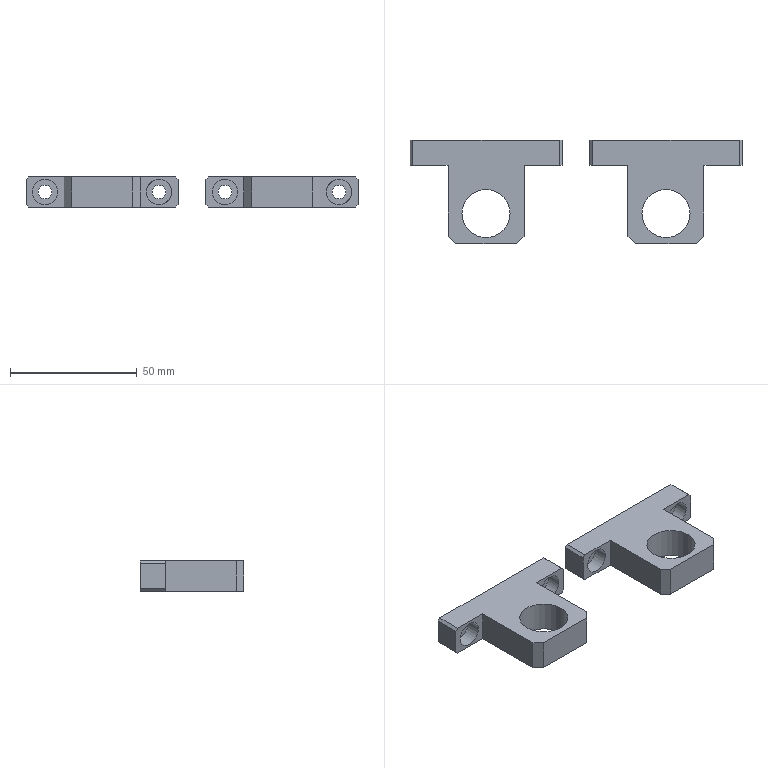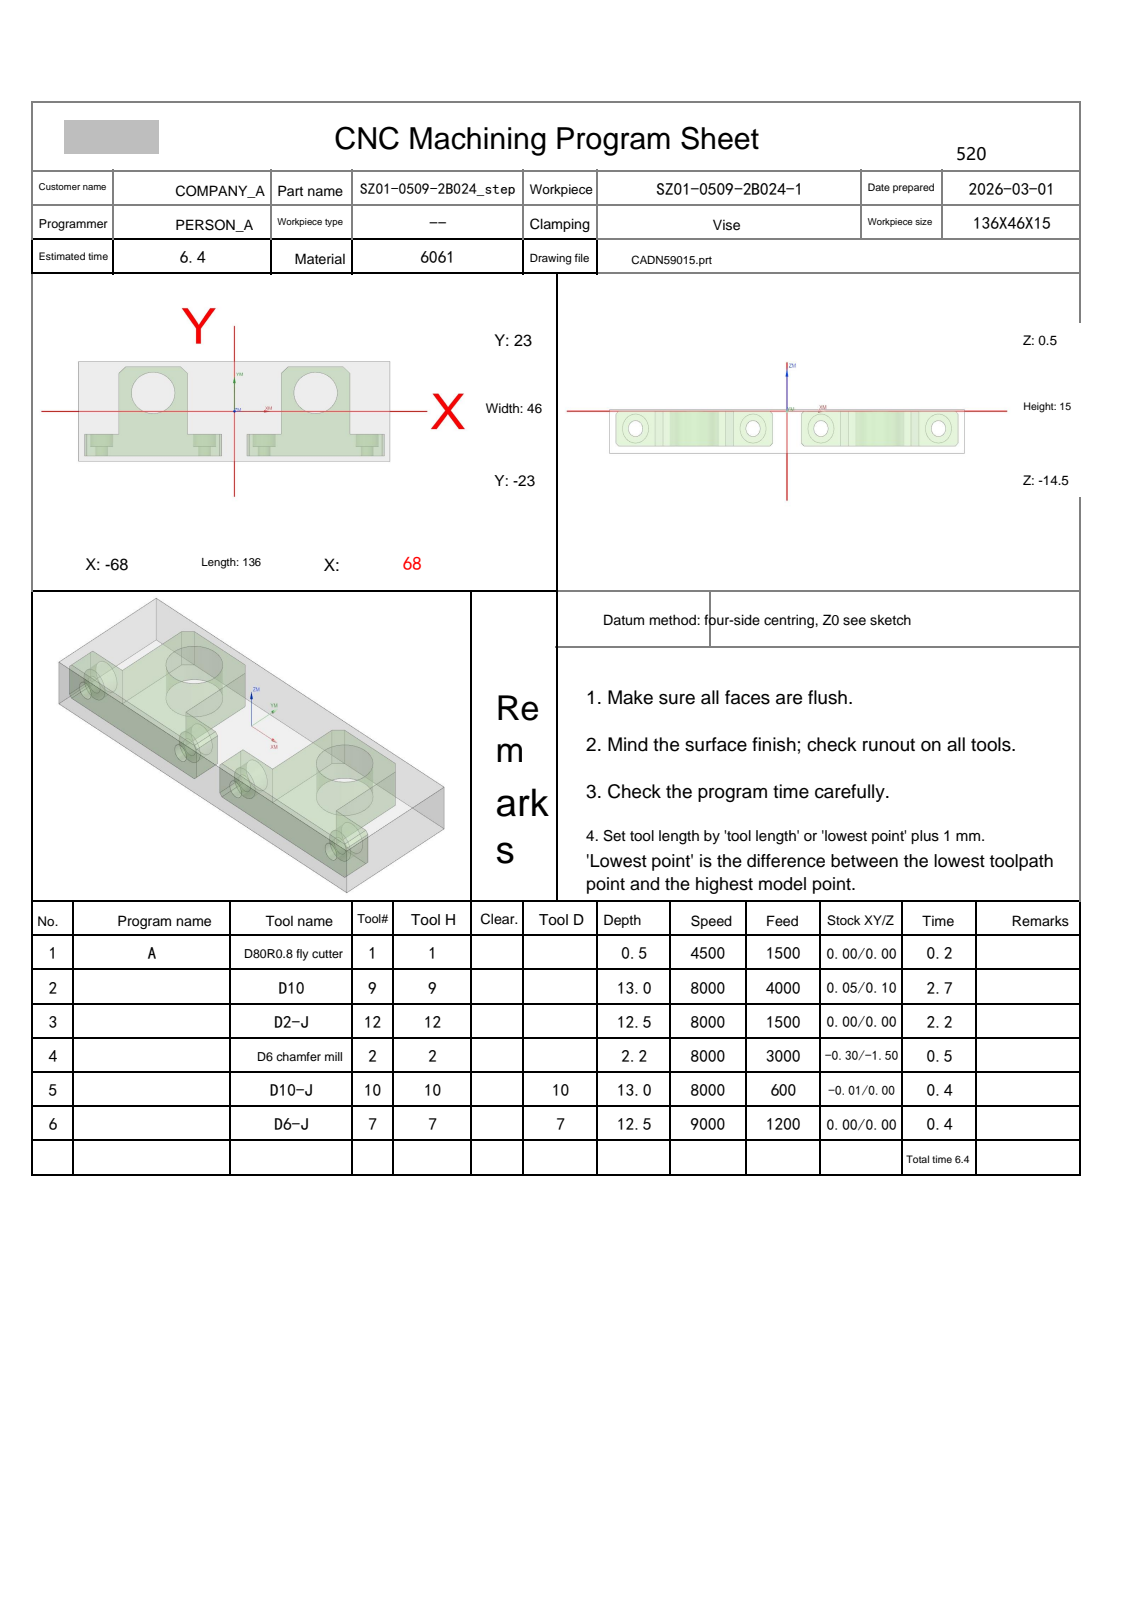NC program | NX | posted by the shop | part box 131 x 41 x 12 mm
Lines 33 to 914 of 8452:
N2 T09 M06
(D10  D=10. R=0. H=09 ce=0.25 di=0.10)
G00 G90 G54 X78.431 Y-9.532 M03 S8000
G43 H09 Z50.
M08
Z-10.
G01 X78.332 Y-9.551 Z-10.625 F4000.
X78.234 Y-9.57 Z-10.872
X78.136 Y-9.588 Z-11.054
X78.038 Y-9.607 Z-11.2
X77.939 Y-9.626 Z-11.323
X77.841 Y-9.644 Z-11.428
X77.743 Y-9.663 Z-11.52
X77.645 Y-9.682 Z-11.6
X77.546 Y-9.7 Z-11.67
X77.448 Y-9.719 Z-11.732
X77.35 Y-9.738 Z-11.786
X77.252 Y-9.756 Z-11.833
X77.153 Y-9.775 Z-11.874
X77.055 Y-9.794 Z-11.908
X76.957 Y-9.812 Z-11.936
X76.859 Y-9.831 Z-11.96
X76.76 Y-9.85 Z-11.977
X76.662 Y-9.869 Z-11.99
X76.564 Y-9.887 Z-11.997
X76.466 Y-9.906 Z-12.
X74.351 Y-10.308
G03 X74. Y-10.567 I.101 J-.505
X73.362 Y-14.375 I12.231 J-4.006
X73.175 Y-21.332 I466.207 J-16.024
G02 X69.942 Y-26.231 I-6.184 J.564
X64.382 Y-27.871 I-6.599 J12.133
X56.567 Y-28.2 I-7.815 J92.472
X55.272 Y-28.191 I0.0 J92.801
G01 X-66.13 Y-28.178
G02 X-71.209 Y-24.969 I.35 J6.178
X-72.866 Y-19.412 I12.012 J6.606
X-73.198 Y-11.704 I89.283 J7.708
X-73.19 Y-10.542 I89.615 J0.0
G01 X-73.178 Y21.13
G02 X-69.969 Y26.209 I6.178 J-.35
X-64.412 Y27.866 I6.606 J-12.012
X-56.704 Y28.198 I7.708 J-89.284
X-55.542 Y28.19 I0.0 J-89.616
G01 X66.15 Y28.176
G02 X71.222 Y24.947 I-.374 J-6.185
X72.868 Y19.389 I-12.074 J-6.599
X73.206 Y11.288 I-97.034 J-8.1
X73.193 Y9.718 I-97.372 J0.0
X73.223 Y2.077 I-972.688 J-7.641
X73.171 Y-8.021 I-972.718 J0.0
G03 X72.526 Y-16.182 I158.167 J-16.601
G01 X72.527 Y-16.395
G02 X72.324 Y-19.878 I-29.998 J0.0
X67.898 Y-25.433 I-7.835 J1.701
X61.268 Y-27.106 I-7.64 J16.307
X51.965 Y-27.41 I-9.303 J141.895
X49.915 Y-27.396 I0.0 J142.199
G01 X-63.987 Y-27.379
G02 X-70.13 Y-23.411 I.587 J7.646
X-72.044 Y-16.849 I14.246 J7.717
X-72.402 Y-8.099 I106.839 J8.75
X-72.392 Y-6.619 I107.197 J0.0
G01 X-72.379 Y18.987
G02 X-68.413 Y25.125 I7.648 J-.591
X-62.168 Y27.003 I7.584 J-13.897
X-53.695 Y27.396 I8.473 J-91.31
X-52.5 Y27.388 I0.0 J-91.702
G01 X63.987 Y27.379
G02 X70.125 Y23.413 I-.591 J-7.648
X72.003 Y17.168 I-13.895 J-7.585
X72.395 Y8.7 I-91.242 J-8.468
X72.388 Y7.5 I-91.635 J0.0
X72.415 Y1.757 I-590.112 J-5.744
X72.352 Y-6.879 I-590.139 J0.0
G03 X71.65 Y-17.634 I789.099 J-56.915
G02 X70.746 Y-20.537 I-9.426 J1.342
G01 X70.57 Y-21.867
X70.045 Y-23.131
X69.211 Y-24.217
X68.124 Y-25.049
X66.859 Y-25.572
G02 X53.023 Y-26.58 I-13.836 J94.442
X52.027 Y-26.575 I0.0 J95.45
G01 X-61.953 Y-26.576
G02 X-65.274 Y-25.768 I.43 J9.002
G01 X-66.859 Y-25.572
X-68.124 Y-25.049
X-69.211 Y-24.217
X-70.045 Y-23.131
X-70.57 Y-21.867
G02 X-71.582 Y-7.951 I95.216 J13.916
X-71.579 Y-7.258 I96.228 J0.0
G01 X-71.575 Y16.961
G02 X-66.822 Y24.292 I8.746 J-.465
X-60.166 Y26.188 I8.154 J-15.995
X-50.795 Y26.602 I9.371 J-105.776
X-49.219 Y26.59 I0.0 J-106.19
G01 X61.968 Y26.575
G02 X69.292 Y21.822 I-.472 J-8.746
X71.177 Y15.251 I-15.881 J-8.113
X71.601 Y5.878 I-103.407 J-9.373
X71.589 Y4.304 I-103.831 J0.0
X71.622 Y.577 I-214.924 J-3.727
X71.462 Y-7.694 I-214.956 J0.0
X70.917 Y-15.927 I-317.939 J16.915
G01 X70.75 Y-16.9
X70.739 Y-20.591
G02 X70.734 Y-17.931 I740.355 J2.66
X70.786 Y-9.213 I740.36 J0.0
G03 X70.973 Y1.153 I-287.439 J10.366
X70.769 Y11.972 I-287.626 J0.0
X69.566 Y19.046 I-25.77 J-.745
X62.385 Y25.338 I-8.77 J-2.765
X55.692 Y25.929 I-6.694 J-37.65
X55.141 Y25.925 I0.0 J-38.24
G01 X49.701 Y25.96
X-50.827 Y25.938
G03 X-51.733 Y25.944 I-.907 J-73.71
X-60.486 Y25.423 I0.0 J-73.716
X-66.63 Y23.268 I1.639 J-14.515
X-70.323 Y17.452 I5.291 J-7.44
X-70.925 Y10.804 I36.408 J-6.648
X-70.921 Y10.289 I37.011 J0.0
X-70.978 Y1.731 I651.006 J-8.558
X-70.84 Y-11.63 I651.062 J0.0
G01 X-70.75 Y-13.67
Y-20.508
Y-10.488
G03 X-70.174 Y-2.848 I-50.43 J7.64
X-70.181 Y-2.016 I-51.006 J0.0
G02 X-70.185 Y.056 I521.372 J2.072
X-70.048 Y12.033 I521.376 J0.0
X-69.175 Y17.625 I19.634 J-.199
X-63.541 Y23.319 I9.252 J-3.521
X-56.373 Y24.868 I8.375 J-21.386
X-49.888 Y25.148 I11.094 J-182.024
G01 X-48.844 Y25.575
X-47.498 Y25.75
X-23.498
G03 X-15.836 Y25.183 I7.662 J51.486
X-15.169 Y25.187 I0.0 J52.053
G01 X21.108 Y25.165
X22.141 Y25.571
X23.502 Y25.75
X47.502
G03 X55.812 Y25.121 I8.791 J60.967
G02 X61.994 Y24.383 I-.07 J-26.825
X68.255 Y18.686 I-2.808 J-9.377
X69.841 Y11.689 I-20.511 J-8.326
X70.171 Y1.353 I-161.858 J-10.336
X70.144 Y-1.584 I-162.187 J0.0
G01 X70.041 Y-7.828
X70.571 Y-9.141
X70.75 Y-10.5
X70.571 Y-9.141
G02 X69.628 Y-5.112 I8.139 J4.029
G01 X69.629 Y-5.056
G02 X69.438 Y6.639 I683.135 J16.984
G03 X68.593 Y15.062 I-42.733 J-.032
X65.546 Y20.951 I-11.68 J-2.311
X59.495 Y23.891 I-7.939 J-8.642
X52.367 Y24.606 I-9.159 J-55.413
G02 X50.426 Y24.826 I.085 J9.434
G01 X50.099 Y25.061
X48.844 Y25.575
G02 X50.69 Y24.663 I-1.998 J-6.365
G03 X54.199 Y23.848 I4.804 J12.726
G02 X60.066 Y22.761 I-3.554 J-35.572
X66.984 Y16.109 I-3.221 J-10.271
X68.456 Y8.601 I-24.166 J-8.637
X68.77 Y-2.859 I-264.069 J-12.979
G03 X69.135 Y-6.654 I20.586 J.063
G01 X70.047 Y-7.875
G02 X68.949 Y-6.346 I6.894 J6.106
X68.234 Y-2.287 I12.715 J4.332
G01 X67.866 Y7.358
G03 X66.546 Y14.9 I-27.424 J-.912
X59.133 Y21.995 I-10.58 J-3.634
X53.397 Y23.316 I-14.209 J-48.594
G02 X51.547 Y23.878 I.966 J6.512
G03 X50.404 Y24.833 I-6.49 J-6.598
G02 X51.798 Y23.654 I-7.538 J-10.322
G03 X54.901 Y22.402 I5.515 J9.195
G02 X60.195 Y20.47 I-5.918 J-24.445
X65.738 Y13.554 I-5.959 J-10.454
X67.057 Y5.848 I-28.689 J-8.879
G03 X67.503 Y-2.521 I339.344 J13.863
X68.266 Y-6.002 I11.413 J.677
X69.212 Y-6.788 I3.867 J3.697
G02 X68.124 Y-5.877 I3.21 J4.942
X67.061 Y-2.591 I7.081 J4.105
X66.47 Y4.858 I92.857 J11.121
G03 X65.214 Y12.577 I-31.943 J-1.236
X57.972 Y20.458 I-11.888 J-3.656
G01 X53.292 Y22.298
X52.941 Y22.483
X51.64 Y23.784
G03 X53.642 Y21.874 I14.828 J13.532
X57.456 Y19.824 I24.045 J40.165
G02 X64.483 Y11.107 I-6.275 J-12.249
X65.712 Y3.298 I-37.08 J-9.835
G03 X66.495 Y-3.256 I46.807 J2.271
X67.452 Y-5.625 I6.665 J1.313
X68.125 Y-5.953 I1.73 J2.696
G01 X68.379 Y-6.148
G03 X67.457 Y-5.666 I-1.885 J-2.482
G02 X66.105 Y-3.2 I3.656 J3.609
X65.225 Y2.036 I29.104 J7.583
G03 X64.123 Y9.539 I-52.704 J-3.906
X57.218 Y18.961 I-14.177 J-3.149
G02 X54.832 Y20.447 I19.818 J34.471
G03 X53.195 Y22.23 I-9.339 J-6.934
G02 X55.215 Y19.957 I-11.166 J-11.96
G03 X58.401 Y17.141 I66.723 J72.254
G02 X63.333 Y8.408 I-11.599 J-12.311
X64.576 Y.707 I-77.667 J-16.487
G03 X65.88 Y-4.262 I17.086 J1.83
X66.693 Y-5.378 I2.512 J.975
G01 X67.598 Y-5.735
G02 X66.486 Y-5.283 I3.324 J9.773
X64.908 Y-2.769 I3.712 J4.081
X63.746 Y2.438 I28.055 J8.995
G03 X62.198 Y9.627 I-41.699 J-5.218
X57.241 Y17.104 I-17.027 J-5.907
G02 X55.624 Y18.73 I83.978 J85.106
G03 X54.926 Y20.308 I-17.041 J-6.584
G02 X55.735 Y18.395 I-16.139 J-7.948
G03 X58.03 Y15.224 I24.329 J15.195
G02 X62.242 Y5.712 I-18.618 J-13.933
G03 X63.657 Y-1.041 I159.818 J29.955
X65.367 Y-4.768 I9.68 J2.187
X66.069 Y-5.325 I1.326 J.95
G01 X66.859 Y-5.429
G02 X65.724 Y-5.21 I.09 J3.511
X63.882 Y-2.879 I2.971 J4.241
X62.27 Y2.59 I24.562 J10.211
G03 X60.077 Y10.169 I-38.367 J-6.997
X56.631 Y15.908 I-29.191 J-13.623
G02 X55.749 Y17.432 I4.421 J3.577
G01 X55.559 Y18.889
X55.821 Y16.912
G03 X57.042 Y14.251 I13.087 J4.392
G02 X61.119 Y3.785 I-32.14 J-18.549
G03 X62.877 Y-2.193 I39.689 J8.423
X64.985 Y-5.166 I6.493 J2.37
X66.057 Y-5.323 I1.2 J4.433
G01 X65.084 Y-5.24
G02 X63.138 Y-3.462 I1.678 J3.79
X61.099 Y1.577 I16.292 J9.523
G03 X58.788 Y8.992 I-68.325 J-17.23
X56.15 Y14.608 I-99.589 J-43.345
G01 X55.749 Y15.649
Y17.409
G03 X55.728 Y16.558 I17.429 J-.851
X55.818 Y14.781 I17.449 J0.0
X57.362 Y10.407 I27.73 J7.326
G02 X60.327 Y1.407 I-95.368 J-36.409
G03 X62.634 Y-3.733 I17.438 J4.739
X64.271 Y-5.23 I3.827 J2.539
G01 X65.174 Y-5.25
G02 X64.807 Y-5.269 I-.367 J3.488
X64.003 Y-5.176 I0.0 J3.507
X61.74 Y-3.023 I2.375 J4.762
X59.452 Y2.312 I20.261 J11.849
G03 X55.987 Y12.216 I-173.547 J-55.152
G01 X55.749 Y12.999
Y15.399
G03 X55.725 Y14.145 I32.92 J-1.254
X55.81 Y11.78 I32.944 J0.0
X57.187 Y6.773 I38.083 J7.784
X59.864 Y-.894 I72.876 J21.136
X62.47 Y-4.71 I9.939 J3.99
X63.379 Y-5.25 I1.617 J1.687
G01 X64.339
G02 X63.918 Y-5.267 I-.421 J5.114
X63.025 Y-5.189 I0.0 J5.131
X60.617 Y-3.094 I2.256 J5.025
X58.01 Y2.374 I19.177 J12.498
X55.749 Y9.479 I94.363 J33.937
G01 Y12.439
G03 X55.726 Y10.8 I59.794 J-1.639
X55.793 Y7.984 I59.817 J0.0
X59.301 Y-2.218 I31.065 J4.979
X62.056 Y-5.176 I7.01 J3.769
X62.911 Y-5.275 I.855 J3.622
X63.341 Y-5.25 I0.0 J3.721
G02 X62.879 Y-5.269 I-.462 J5.785
X61.937 Y-5.192 I0.0 J5.803
X59.319 Y-2.974 I2.344 J5.422
X56.249 Y3.636 I19.456 J13.054
G01 X55.749 Y5.411
Y8.531
G03 X55.726 Y6.853 I61.797 J-1.678
X55.792 Y3.995 I61.819 J0.0
X59.379 Y-3.947 I15.561 J2.247
X61.095 Y-5.239 I3.86 J3.341
G01 X62.276 Y-5.25
G02 X61.786 Y-5.269 I-.489 J6.504
X60.793 Y-5.192 I0.0 J6.522
X58.085 Y-2.941 I2.349 J5.579
X55.75 Y1.923 I12.574 J9.03
G01 X55.749 Y4.563
G03 X55.726 Y3.244 I36.451 J-1.319
X55.804 Y.848 I36.475 J0.0
X59.294 Y-4.891 I9.243 J1.689
X59.997 Y-5.25 I1.435 J1.945
G01 X61.117
G02 X60.594 Y-5.273 I-.523 J5.928
X59.649 Y-5.198 I0.0 J5.951
X56.981 Y-2.964 I2.169 J5.3
X55.75 Y-.509 I7.416 J5.256
G01 Y1.411
G03 X55.728 Y.467 I20.777 J-.944
X55.795 Y-1.196 I20.799 J0.0
X58.791 Y-5.229 I5.838 J1.208
G01 X59.939 Y-5.25
G02 X59.475 Y-5.27 I-.464 J5.379
X58.525 Y-5.186 I0.0 J5.399
X55.75 Y-2.143 I1.94 J4.557
G01 Y-.783
G03 X55.727 Y-1.441 I9.704 J-.658
X55.809 Y-2.694 I9.727 J0.0
X57.863 Y-5.234 I3.857 J1.019
G01 X58.836 Y-5.25
G02 X58.438 Y-5.269 I-.397 J4.269
X57.595 Y-5.185 I0.0 J4.287
X55.75 Y-3.223 I1.223 J2.999
G01 Y-2.263
G03 X55.728 Y-2.724 I4.868 J-.461
X55.841 Y-3.768 I4.89 J0.0
X57.126 Y-5.231 I2.453 J.859
G01 X57.945 Y-5.25
G02 X57.606 Y-5.271 I-.339 J2.707
X56.858 Y-5.167 I0.0 J2.728
X55.75 Y-3.933 I.806 J1.838
G01 Y-3.373
G03 X55.725 Y-3.675 I1.823 J-.302
X56.483 Y-5.166 I1.848 J0.0
X57.015 Y-5.264 I.532 J1.403
X57.219 Y-5.25 I0.0 J1.501
G02 X56.968 Y-5.275 I-.251 J1.247
X55.75 Y-4.369 I0.0 J1.272
G01 Y-3.969
G03 X55.727 Y-4.203 I1.163 J-.234
X56.292 Y-5.213 I1.186 J0.0
G01 X56.734 Y-5.25
X56.545 Y-5.271
G02 X55.818 Y-4.853 I0.0 J.84
X55.751 Y-4.588 I.482 J.265
X56.301 Y-4.038 I.55 J0.0
X56.729 Y-4.243 I0.0 J-.55
X56.929 Y-4.696 I-.412 J-.453
X56.878 Y-4.941 I-.612 J0.0
X56.385 Y-5.245 I-.493 J.248
G01 X56.278 Y-5.234
G02 X55.729 Y-4.572 I.124 J.662
G01 X55.75 Y-4.404
G02 X56.021 Y-3.959 I.504 J-.003
G01 X56.544 Y-3.69
X58.298 Y-2.789 Z-11.9
X59.363 Y-2.241
X59.436 Y-2.21
X59.513 Y-2.192
X59.592 Y-2.185
X67.964
X68.18 Y-2.192
X68.396 Y-2.212
X68.611 Y-2.244
X68.823 Y-2.29
X69.032 Y-2.348
X69.237 Y-2.419
X69.437 Y-2.502
X69.632 Y-2.597
X69.821 Y-2.703
X70.003 Y-2.821
X70.177 Y-2.949
X70.344 Y-3.088
X70.502 Y-3.237
X73.328 Y-6.063
X73.477 Y-6.221
X73.616 Y-6.388
X73.744 Y-6.562
X73.862 Y-6.744
X73.969 Y-6.933
X74.064 Y-7.128
X74.147 Y-7.329
X74.217 Y-7.534
X74.276 Y-7.742
X74.321 Y-7.954
X74.354 Y-8.169
X74.373 Y-8.385
X74.38 Y-8.602
Y-23.146
X74.372 Y-23.333
X74.35 Y-23.52
X74.313 Y-23.704
X74.262 Y-23.885
X74.196 Y-24.061
X74.117 Y-24.232
X74.024 Y-24.395
X73.919 Y-24.551
X73.802 Y-24.698
X73.673 Y-24.836
X73.535 Y-24.962
X73.386 Y-25.077
X69.342 Y-27.968
X69.275 Y-28.008
X69.204 Y-28.038
X69.128 Y-28.055
X69.051 Y-28.061
X68.974 Y-28.055
X68.898 Y-28.037
X68.826 Y-28.008
X68.76 Y-27.968
X68.331 Y-27.661
X66.728 Y-26.514 Z-12.
X65.724 Y-25.803
X65.5 Y-25.75
X3.682 Y-25.774
X-59.749 Y-25.787
G03 X-63.515 Y-25.736 I-3.766 J-140.302
X-65.448 Y-25.75 I0.0 J-140.353
G01 X-5.502
G02 X1.947 Y-25.165 I7.449 J-47.095
X3.199 Y-25.181 I0.0 J-47.681
G01 X4.141 Y-25.571
X5.498 Y-25.75
X4.141 Y-25.571
G03 X.069 Y-24.642 I-4.072 J-8.461
X-.135 Y-24.644 I0.0 J-9.39
X-.855 Y-24.622 I-.72 J-11.256
X-2.434 Y-24.733 I0.0 J-11.279
G01 X-2.875 Y-25.047
X-4.141 Y-25.571
X-2.875 Y-25.047
G02 X-1.229 Y-24.372 I1.82 J-2.096
X.205 Y-24.241 I1.434 J-7.777
X2.124 Y-24.478 I0.0 J-7.908
G01 X2.949 Y-25.077
G03 X1.701 Y-24.228 I-5.954 J-7.409
X-.255 Y-23.865 I-1.956 J-5.083
X-1.582 Y-24.029 I0.0 J-5.446
G01 X-2.486 Y-24.748
G03 X-1.634 Y-24.031 I-2.311 J3.61
G02 X.088 Y-23.614 I1.722 J-3.346
X1.505 Y-23.891 I0.0 J-3.763
G03 X2.042 Y-24.407 I3.361 J2.958
G02 X1.505 Y-23.855 I1.395 J1.892
G03 X-.144 Y-23.346 I-1.649 J-2.416
X-1.251 Y-23.563 I0.0 J-2.925
G01 X-1.749 Y-24.162
G02 X-1.078 Y-23.423 I2.078 J-1.211
X.011 Y-23.158 I1.089 J-2.112
X1.23 Y-23.495 I0.0 J-2.376
G01 X1.595 Y-23.962
G03 X-.094 Y-22.955 I-1.689 J-.914
X-.951 Y-23.157 I0.0 J-1.921
G01 X-1.325 Y-23.61
G02 X-.001 Y-22.819 I1.325 J-.714
X.48 Y-22.898 I0.0 J-1.505
X1.207 Y-23.456 I-.203 J-1.018
G03 X-.056 Y-22.684 I-1.264 J-.647
X-.809 Y-22.899 I0.0 J-1.42
G01 X-1.002 Y-23.188
G02 X-.074 Y-22.58 I.928 J-.403
G01 X.123 Y-22.599
X.162 Y-22.598
G02 X.953 Y-23.125 I0.0 J-.858
G03 X-.004 Y-22.456 I-.958 J-.351
X-.237 Y-22.483 I0.0 J-1.02
X-.924 Y-23.054 I.03 J-.734
G02 X-.034 Y-22.377 I.89 J-.247
X.246 Y-22.421 I0.0 J-.924
X.874 Y-22.933 I-.08 J-.739
G03 X-.012 Y-22.273 I-.885 J-.265
X-.757 Y-22.651 I0.0 J-.924
G01 X-.849 Y-22.873
G02 X.007 Y-22.209 I.856 J-.22
X.729 Y-22.584 I0.0 J-.883
G01 X.79 Y-22.731
G03 X-.008 Y-22.126 I-.798 J-.223
X-.684 Y-22.474 I0.0 J-.829
G01 X-.745 Y-22.622
G02 X-.002 Y-22.069 I.743 J-.223
X.724 Y-22.571 I0.0 J-.776
G03 X.006 Y-21.995 I-.718 J-.159
X-.685 Y-22.477 I0.0 J-.736
G02 X-.004 Y-21.945 I.681 J-.17
X.633 Y-22.352 I0.0 J-.702
G03 X.001 Y-21.882 I-.632 J-.19
X-.622 Y-22.324 I0.0 J-.66
G02 X-.004 Y-21.84 I.618 J-.153
X.576 Y-22.215 I0.0 J-.637
G03 X.001 Y-21.784 I-.576 J-.169
X-.569 Y-22.198 I0.0 J-.6
G02 X0.0 Y-21.711 I.569 J-.09
X.569 Y-22.198 I0.0 J-.576
G01 X.601 Y-22.473
G02 X.022 Y-25.82 I-165.263 J26.853
G01 X-.067 Y-25.947
X-.138 Y-26.018 Z-11.997
X-.209 Y-26.089 Z-11.99
X-.279 Y-26.16 Z-11.977
X-.35 Y-26.23 Z-11.96
X-.421 Y-26.301 Z-11.936
X-.491 Y-26.372 Z-11.908
X-.562 Y-26.442 Z-11.874
X-.633 Y-26.513 Z-11.833
X-.704 Y-26.584 Z-11.786
X-.774 Y-26.655 Z-11.732
X-.845 Y-26.725 Z-11.67
X-.916 Y-26.796 Z-11.6
X-.986 Y-26.867 Z-11.52
X-1.057 Y-26.937 Z-11.428
X-1.128 Y-27.008 Z-11.323
X-1.199 Y-27.079 Z-11.2
X-1.269 Y-27.15 Z-11.054
X-1.34 Y-27.22 Z-10.872
X-1.411 Y-27.291 Z-10.625
X-1.481 Y-27.362 Z-10.
G00 Z50.
X-20.845 Y29.605
Z-10.
G01 X-20.908 Y29.528 Z-10.625
X-20.972 Y29.45 Z-10.872
X-21.035 Y29.372 Z-11.054
X-21.098 Y29.295 Z-11.2
X-21.161 Y29.217 Z-11.323
X-21.224 Y29.139 Z-11.428
X-21.287 Y29.062 Z-11.52
X-21.35 Y28.984 Z-11.6
X-21.413 Y28.906 Z-11.67
X-21.476 Y28.829 Z-11.732
X-21.539 Y28.751 Z-11.786
X-21.602 Y28.674 Z-11.833
X-21.665 Y28.596 Z-11.874
X-21.728 Y28.518 Z-11.908
X-21.791 Y28.441 Z-11.936
X-21.854 Y28.363 Z-11.96
X-21.917 Y28.285 Z-11.977
X-21.98 Y28.208 Z-11.99
X-22.043 Y28.13 Z-11.997
X-22.106 Y28.052 Z-12.
X-22.174 Y27.934
X-22.214 Y27.803
X-22.448 Y26.107
X-22.453 Y26.039
G03 X-22.141 Y25.571 I.507 J0.0
X-18.015 Y24.627 I4.635 J10.762
X-8.539 Y24.343 I9.476 J158.027
X-6.171 Y24.36 I0.0 J158.311
G01 X19.349 Y24.378
X19.41 Y24.377
G03 X20.18 Y24.513 I0.0 J2.248
G02 X21.245 Y25.2 I2.329 J-2.443
G03 X20.116 Y24.465 I1.398 J-3.379
G02 X17.375 Y23.911 I-2.9 J7.299
X8.655 Y23.7 I-8.72 J180.058
X5.989 Y23.72 I0.0 J180.269
X-.188 Y23.697 I-6.177 J822.824
X-14.733 Y23.825 I0.0 J822.847
X-19.994 Y24.385 I.165 J26.575
G01 X-20.875 Y25.047
X-21.392 Y25.261
G02 X-20.052 Y24.415 I-1.421 J-3.736
G03 X-17.182 Y23.443 I3.518 J5.665
X-9.435 Y22.945 I7.747 J60.059
X-8.688 Y22.95 I0.0 J60.557
X.874 Y22.898 I9.563 J887.517
X14.641 Y23.005 I0.0 J887.568
X19.026 Y23.519 I-.006 J19.017
X19.789 Y24.213 I-1.817 J2.765
G01 X20.17 Y24.506
G03 X19.125 Y23.55 I5.183 J-6.713
G02 X16.159 Y22.653 I-3.484 J6.173
X8.998 Y22.291 I-7.161 J70.659
X8.121 Y22.297 I0.0 J71.021
X1.222 Y22.257 I-6.899 J607.759
X-12.156 Y22.405 I0.0 J607.798
X-18.217 Y23.148 I.277 J27.331
X-19.049 Y23.473 I1.78 J5.783
G01 X-19.977 Y24.357
X-18.787 Y23.239
G03 X-15.402 Y22.073 I4.371 J7.196
X-7.196 Y21.515 I8.206 J60.033
X-6.599 Y21.518 I0.0 J60.592
X.768 Y21.459 I7.367 J459.466
X12.516 Y21.609 I0.0 J459.525
X17.837 Y22.386 I-.167 J19.741
G01 X18.091 Y22.515
X19.165 Y23.59
G02 X17.803 Y22.284 I-11.131 J10.252
X14.185 Y21.247 I-4.381 J8.454
X5.885 Y20.843 I-8.3 J84.987
X4.61 Y20.852 I0.0 J85.392
X.21 Y20.818 I-4.4 J285.684
X-11.424 Y21.055 I0.0 J285.718
X-17.278 Y22.031 I.636 J21.85
G01 X-17.876 Y22.301
X-18.951 Y23.376
G03 X-17.263 Y21.809 I8.544 J7.514
X-13.263 Y20.601 I5.228 J10.083
X-4.318 Y20.067 I8.945 J74.587
X-3.571 Y20.07 I0.0 J75.121
X1.131 Y20.024 I4.702 J240.393
X11.401 Y20.244 I0.0 J240.439
X16.655 Y21.162 I-.581 J18.823
G01 X16.842 Y21.267
X18.087 Y22.511
G02 X16.566 Y21.037 I-28.047 J27.416
X12.971 Y19.911 I-4.561 J8.256
X4.706 Y19.422 I-8.265 J69.648
X3.873 Y19.427 I0.0 J70.137
X.232 Y19.392 I-3.641 J188.298
X-10.325 Y19.688 I0.0 J188.334
X-16.08 Y20.771 I.974 J21.005
X-16.787 Y21.211 I.327 J1.314
G01 X-17.748 Y22.173
X-16.319 Y20.72
G03 X-12.6 Y19.351 I5.028 J7.924
X-3.882 Y18.667 I8.718 J55.245
G01 X-3.693
G03 X.853 Y18.605 I4.546 J166.377
X10.161 Y18.866 I0.0 J166.44
X15.386 Y19.865 I-.831 J18.502
X16.008 Y20.196 I-1.273 J3.141
G01 X16.789 Y21.213
G02 X15.636 Y19.853 I-5.692 J3.653
X11.988 Y18.59 I-4.805 J7.979
X3.696 Y18.009 I-8.292 J58.951
X3.139 Y18.012 I0.0 J59.531
X.092 Y17.974 I-3.047 J121.346
X-9.967 Y18.391 I0.0 J121.384
X-15.3 Y19.662 I1.237 J17.017
X-15.953 Y20.125 I.485 J1.377
G01 X-16.635 Y21.014
G03 X-15.633 Y19.699 I22.221 J15.903
X-12.329 Y18.192 I4.834 J6.222
X-4.112 Y17.296 I8.538 J40.151
X.693 Y17.193 I4.805 J112.243
X9.727 Y17.557 I0.0 J112.346
X14.666 Y18.722 I-1.142 J15.887
X15.656 Y19.406 I-.852 J2.291
G01 X15.953 Y20.125
G02 X15.451 Y19.095 I-2.955 J.805
X12.53 Y17.595 I-4.346 J4.869
X5.25 Y16.685 I-7.721 J32.172
X.555 Y16.573 I-4.696 J98.966
X-9.033 Y17.038 I0.0 J99.078
X-14.375 Y18.411 I1.498 J16.911
X-15.615 Y19.308 I1.343 J3.162
G01 X-15.921 Y20.048
G03 X-14.021 Y17.846 I3.301 J.928
X-8.826 Y16.353 I6.88 J14.154
X.737 Y15.803 I9.564 J82.936
X4.71 Y15.898 I0.0 J83.486
X12.251 Y16.849 I-.358 J33.199
X15.284 Y18.388 I-1.633 J6.977
X15.429 Y18.859 I-1.207 J.628
G01 X15.643 Y19.376
G03 X15.368 Y18.473 I2.334 J-1.205
G02 X13.342 Y16.864 I-3.513 J2.342
X7.383 Y15.506 I-7.157 J17.654
X.514 Y15.197 I-6.87 J76.132
X-8.55 Y15.736 I0.0 J76.441
X-14.056 Y17.375 I1.678 J15.699
X-15.365 Y18.493 I1.482 J3.062
G03 X-15.582 Y19.228 I-2.76 J-.415
G02 X-15.366 Y18.423 I-2.037 J-.977
G03 X-13.547 Y16.665 I3.579 J1.882
X-7.995 Y14.994 I7.421 J14.596
X.573 Y14.441 I8.568 J66.172
X8.698 Y14.938 I0.0 J66.725
X13.89 Y16.523 I-1.638 J14.657
X15.259 Y17.721 I-1.913 J3.567
G01 X15.397 Y18.615
G02 X15.169 Y17.468 I-3.36 J.072
X12.64 Y15.523 I-4.386 J3.086
X6.206 Y14.102 I-7.745 J19.798
X.504 Y13.835 I-5.702 J60.585
X-8.511 Y14.506 I0.0 J60.853
X-13.795 Y16.315 I2.078 J14.693
X-15.276 Y17.756 I2. J3.536
G01 X-15.384 Y18.514
G03 X-14.124 Y16.134 I2.918 J.021
X-9.493 Y14.078 I6.956 J9.426
X-.271 Y13.105 I9.222 J43.226
X.478 Y13.112 I0.0 J44.199
X1.429 Y13.101 I.952 J42.012
X9.987 Y13.981 I0.0 J42.023
X14.407 Y15.961 I-2.122 J10.663
X15.25 Y17.056 I-1.233 J1.821
G01 X15.292 Y17.819
X15.24 Y16.897
G02 X13.507 Y14.959 I-3.65 J1.52
X7.875 Y13.051 I-7.546 J13.006
X.43 Y12.496 I-7.445 J49.694
X-8.554 Y13.306 I0.0 J50.249
X-13.815 Y15.386 I2.347 J13.627
X-15.228 Y16.955 I2.42 J3.6
G01 X-15.281 Y17.736
G03 X-15.198 Y16.711 I10.057 J.297
X-13.188 Y14.475 I4.328 J1.869
X-7.372 Y12.42 I8.2 J13.951
X.446 Y11.761 I7.818 J46.065
X8.656 Y12.488 I0.0 J46.723
X13.816 Y14.523 I-2.295 J13.38
X15.241 Y16.131 I-2. J3.207
G01 X15.25 Y16.983
G02 X15.269 Y16.619 I-3.559 J-.364
X15.179 Y15.821 I-3.577 J0.0
X12.934 Y13.557 I-4.57 J2.287
X6.824 Y11.639 I-8.133 J15.217
X.452 Y11.179 I-6.372 J43.865
X-8.472 Y12.086 I0.0 J44.325
X-13.853 Y14.433 I2.603 J13.311
X-15.25 Y16.221 I2.178 J3.142
G01 Y17.021
G03 X-15.274 Y16.611 I3.498 J-.41
X-15.126 Y15.602 I3.522 J0.0
X-12.653 Y13.086 I5.198 J2.636
X-6.187 Y10.976 I8.865 J16.202
X.401 Y10.455 I6.588 J41.454
X8.517 Y11.247 I0.0 J41.974
X13.83 Y13.499 I-2.542 J13.389
X15.243 Y15.182 I-2.229 J3.307
G01 X15.25 Y16.104
G02 X15.268 Y15.709 I-4.364 J-.395
X15.186 Y14.866 I-4.382 J0.0
X13.008 Y12.519 I-4.724 J2.199
X6.825 Y10.394 I-8.43 J14.473
X.436 Y9.878 I-6.389 J39.327
X-8.473 Y10.887 I0.0 J39.843
X-13.913 Y13.46 I2.876 J13.122
X-15.25 Y15.255 I2.437 J3.21
G01 Y16.135
G03 X-15.274 Y15.704 I3.866 J-.431
X-15.103 Y14.564 I3.89 J0.0
X-12.528 Y11.917 I5.569 J2.842
X-5.71 Y9.652 I9.281 J16.546
X.387 Y9.164 I6.097 J37.799
X8.461 Y10.025 I0.0 J38.287
X13.887 Y12.478 I-2.757 J13.322
X15.239 Y14.14 I-2.69 J3.571
G01 X15.25 Y15.162
G02 X15.268 Y14.738 I-4.928 J-.423
X15.187 Y13.843 I-4.946 J0.0
X12.982 Y11.393 I-4.932 J2.222
X6.563 Y9.109 I-8.791 J14.547
X.426 Y8.594 I-6.137 J36.288
X-8.418 Y9.673 I0.0 J36.803
X-13.824 Y12.32 I3.201 J13.38
X-15.25 Y14.249 I2.681 J3.474
G01 Y15.129
G03 X-15.273 Y14.695 I4.018 J-.434
X-15.102 Y13.532 I4.041 J0.0
X-12.418 Y10.732 I5.858 J2.929
X-5.357 Y8.35 I9.604 J16.812
X.373 Y7.88 I5.73 J34.697
X8.731 Y8.888 I0.0 J35.167
X14.063 Y11.538 I-3.01 J12.747
X15.234 Y13.057 I-3.112 J3.608
G01 X15.25 Y14.19
G02 X15.269 Y13.729 I-5.703 J-.462
X15.191 Y12.788 I-5.722 J0.0
X12.984 Y10.267 I-5.076 J2.217
X6.38 Y7.84 I-9.086 J14.523
X.419 Y7.319 I-5.961 J33.88
X-8.511 Y8.498 I0.0 J34.401
X-13.955 Y11.348 I3.402 J13.125
X-15.25 Y13.191 I2.849 J3.378
G01 Y14.151
G03 X-15.273 Y13.687 I4.592 J-.464
X-15.12 Y12.507 I4.615 J0.0
X-12.581 Y9.704 I5.845 J2.743
X-5.623 Y7.155 I9.764 J15.884
X.361 Y6.611 I5.984 J32.639
X8.809 Y7.705 I0.0 J33.183
X14.164 Y10.518 I-3.184 J12.561
X15.25 Y12.052 I-2.297 J2.779
G01 Y13.092
G02 X15.27 Y12.626 I-5.447 J-.466
X15.188 Y11.68 I-5.466 J0.0
X13.006 Y9.139 I-5.173 J2.235
X6.41 Y6.611 I-9.265 J14.301
X.41 Y6.054 I-6. J32.032
X-8.612 Y7.327 I0.0 J32.589
X-14.033 Y10.312 I3.603 J12.96
X-15.25 Y12.105 I2.921 J3.292
G01 Y13.065
G03 X-15.274 Y12.595 I4.531 J-.47
X-15.113 Y11.392 I4.555 J0.0
X-12.494 Y8.498 I6.044 J2.836
X-5.109 Y5.828 I10.091 J16.363
X.359 Y5.351 I5.468 J31.139
X8.903 Y6.527 I0.0 J31.616
X14.194 Y9.414 I-3.389 J12.504
X15.25 Y10.942 I-2.307 J2.724
G01 Y11.982
G02 X15.269 Y11.518 I-5.849 J-.464
X15.192 Y10.572 I-5.868 J0.0
X12.887 Y7.897 I-5.366 J2.293
X5.903 Y5.285 I-9.571 J14.944
X.402 Y4.794 I-5.501 J30.605
X-8.857 Y6.205 I0.0 J31.096
X-14.217 Y9.371 I3.76 J12.488
X-15.25 Y11. I2.888 J2.973
G01 Y11.96
G03 X-15.274 Y11.49 I4.625 J-.47
X-15.11 Y10.266 I4.649 J0.0
X-12.467 Y7.317 I6.183 J2.883
X-4.945 Y4.564 I10.266 J16.395
X.358 Y4.098 I5.304 J29.951
X9.017 Y5.356 I0.0 J30.417
X14.273 Y8.346 I-3.526 J12.313
X15.25 Y9.804 I-2.299 J2.598
G01 Y10.924
G02 X15.27 Y10.426 I-6.23 J-.498
X15.19 Y9.431 I-6.25 J0.0
X12.966 Y6.784 I-5.355 J2.242
X6.149 Y4.1 I-9.637 J14.476
X.396 Y3.544 I-5.753 J29.506
X-8.971 Y5.041 I0.0 J30.061
X-14.165 Y8.17 I3.998 J12.515
X-15.25 Y9.866 I3.043 J3.141
G01 Y10.906
G03 X-15.273 Y10.408 I5.271 J-.498
X-15.127 Y9.17 I5.295 J0.0
X-12.549 Y6.201 I6.182 J2.764
X-5.069 Y3.352 I10.383 J16.015
X.35 Y2.851 I5.419 J29.034
X9.136 Y4.188 I0.0 J29.535
X14.322 Y7.236 I-3.669 J12.175
X15.25 Y8.644 I-2.413 J2.601
G01 Y9.764
G02 X15.27 Y9.27 I-6.281 J-.494
X15.19 Y8.273 I-6.301 J0.0
X13.047 Y5.666 I-5.37 J2.23
X6.061 Y2.854 I-9.817 J14.303
X.39 Y2.3 I-5.672 J28.737
X-9.02 Y3.852 I0.0 J29.291
X-14.214 Y7.063 I4.119 J12.472
X-15.25 Y8.709 I3.166 J3.141
G01 Y9.749
G03 X-15.269 Y9.26 I6.351 J-.489
X-15.173 Y8.157 I6.37 J0.0
X-12.935 Y5.308 I5.809 J2.259
X-5.794 Y2.266 I10.384 J14.473
X.337 Y1.607 I6.131 J28.196
X9.259 Y3.021 I0.0 J28.854
X14.383 Y6.132 I-3.785 J12.01
X15.25 Y7.47 I-2.408 J2.51
G01 Y8.59
G02 X15.27 Y8.097 I-6.051 J-.494
X15.187 Y7.096 I-6.072 J0.0
X12.932 Y4.397 I-5.522 J2.321
X5.775 Y1.571 I-9.952 J14.732
X.383 Y1.06 I-5.392 J28.168
X-9.073 Y2.664 I0.0 J28.68
X-14.344 Y6.04 I4.114 J12.226
X-15.25 Y7.549 I3.093 J2.884
G01 Y8.589
G03 X-15.273 Y8.091 I5.299 J-.498
X-15.125 Y6.845 I5.322 J0.0
X-12.508 Y3.803 I6.352 J2.819
X-4.691 Y.824 I10.645 J16.182
X.351 Y.369 I5.043 J27.729
X9.384 Y1.855 I0.0 J28.184
X14.45 Y5.028 I-3.878 J11.826
X15.25 Y6.304 I-2.379 J2.38
G01 Y7.424
G02 X15.268 Y6.934 I-6.619 J-.49
X15.193 Y5.938 I-6.638 J0.0
X12.921 Y3.196 I-5.581 J2.312
X5.761 Y.342 I-10.022 J14.733
X.377 Y-.179 I-5.385 J27.576
X-9.266 Y1.528 I0.0 J28.097
X-14.401 Y4.929 I4.224 J11.951
X-15.25 Y6.376 I3.236 J2.873
G01 Y7.416
G03 X-15.274 Y6.914 I5.201 J-.502